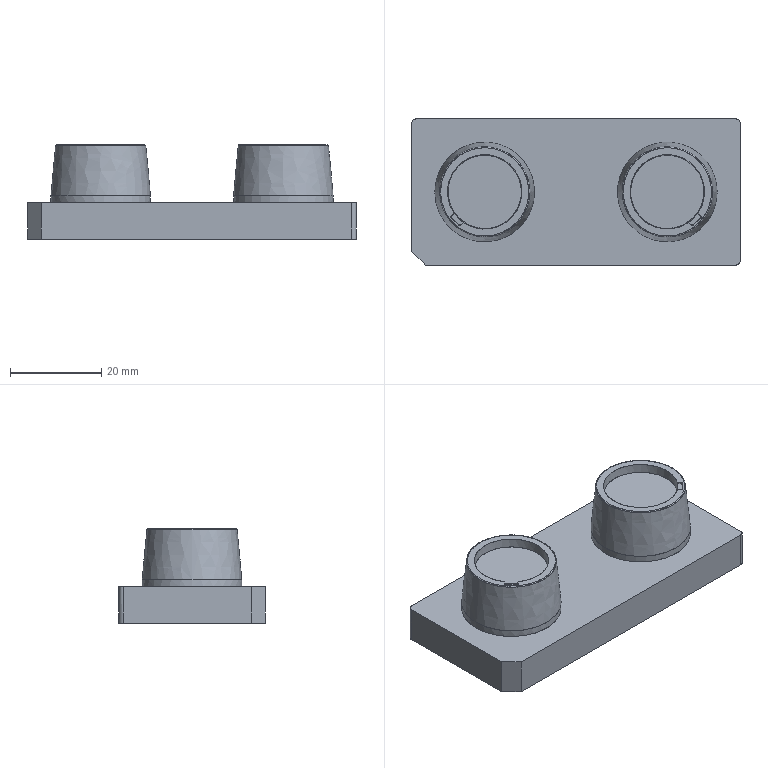NC program | PowerMill | posted with a generic post | part box 72 x 32 x 20.655 mm
Lines 24483 to 25676 of 315359:
N24580 M6
N24581 S8500 M03
N24582 G00 G90 X0.0 Y0.0
N24583 G43 Z11.805 H3
N24584
N24585 G05 P10000 R8
N24586 X-23.5434 Y-20.1661
N24587 Z0.9345
N24588 G01 Z-0.2655 F360.0
N24589 X-22.6227 Y-14.9721 F600.0
N24590 X-5.0883 Y-2.9309
N24591 X-5.0416 Y-2.7032
N24592 X-4.9592 Y-2.1939
N24593 X-4.9004 Y-1.7482
N24594 X-4.8405 Y-1.1118
N24595 X-4.8069 Y-0.4795
N24596 G03 X-4.8205 Y0.7968 I-16.4609 J0.4622
N24597 G01 X-4.8412 Y1.1159
N24598 X-4.9006 Y1.7482
N24599 X-4.9425 Y2.0766
N24600 X-4.9915 Y2.4041
N24601 X-27.6316 Y-13.1433
N24602 X-27.8712 Y-13.0029
N24603 X-28.1923 Y-12.8042
N24604 X-28.5435 Y-12.5711
N24605 X-28.8264 Y-12.374
N24606 X-29.1441 Y-12.1435
N24607 X-29.4654 Y-11.89
N24608 X-29.7833 Y-11.6323
N24609 X-30.1672 Y-11.2986
N24610 X-30.4178 Y-11.0676
N24611 X-30.7384 Y-10.7587
N24612 X-31.1708 Y-10.3051
N24613 X-6.3695 Y6.7262
N24614 X-6.4268 Y6.8444
N24615 X-6.7682 Y7.4807
N24616 X-7.1481 Y8.1163
N24617 X-7.3552 Y8.4344
N24618 X-7.5735 Y8.7524
N24619 X-7.8245 Y9.101
N24620 X-8.0467 Y9.3891
N24621 X-8.3036 Y9.7074
N24622 X-8.5753 Y10.0256
N24623 X-8.8287 Y10.306
N24624 X-33.6284 Y-6.7244
N24625 X-33.73 Y-6.523
N24626 X-33.8779 Y-6.2034
N24627 X-34.1425 Y-5.5711
N24628 X-34.2642 Y-5.252
N24629 X-34.3769 Y-4.9336
N24630 X-34.5563 Y-4.3756
N24631 X-34.7532 Y-3.6623
N24632 X-34.8275 Y-3.3423
N24633 X-34.8968 Y-3.0212
N24634 X-35.0084 Y-2.4035
N24635 X-12.3682 Y13.1439
N24636 X-12.4756 Y13.208
N24637 X-13.0644 Y13.526
N24638 X-13.5529 Y13.7649
N24639 X-13.8711 Y13.9097
N24640 X-14.1896 Y14.0457
N24641 X-14.5066 Y14.172
N24642 X-14.826 Y14.2925
N24643 X-15.145 Y14.4034
N24644 X-15.781 Y14.6032
N24645 X-16.0995 Y14.69
N24646 X-16.7366 Y14.8468
N24647 X-17.3784 Y14.9718
N24648 X-34.9156 Y2.9287
N24649 G00 Z4.0045
N24650 G01 X19.87 Y-20.4718 F10000.0
N24651 G00 Z0.9345
N24652 G01 Z-0.2655 F360.0
N24653 X19.9021 Y-15.1969 F600.0
N24654 X35.195 Y-0.4115
N24655 X35.1988 Y0.161
N24656 X35.1803 Y0.7972
N24657 X35.1585 Y1.1157
N24658 X35.0999 Y1.7525
N24659 X35.0117 Y2.3882
N24660 X34.9565 Y2.7065
N24661 X34.8735 Y3.1296
N24662 X34.7517 Y3.6605
N24663 X34.6699 Y3.9799
N24664 X34.5807 Y4.2974
N24665 X34.4825 Y4.6158
N24666 X34.4005 Y4.861
N24667 X14.657 Y-14.2273
N24668 X14.1865 Y-14.0444
N24669 X13.55 Y-13.7657
N24670 X13.0606 Y-13.5243
N24671 X12.5985 Y-13.2762
N24672 X12.2798 Y-13.0928
N24673 X11.9601 Y-12.8975
N24674 X11.6438 Y-12.6968
N24675 X11.3254 Y-12.4822
N24676 X11.0068 Y-12.2536
N24677 X10.6944 Y-12.0177
N24678 X32.3248 Y8.895
N24679 X32.1975 Y9.0709
N24680 X31.9539 Y9.3894
N24681 X31.6953 Y9.7073
N24682 X31.4242 Y10.0254
N24683 X31.1379 Y10.3444
N24684 X30.7362 Y10.758
N24685 X30.5094 Y10.9804
N24686 X30.0993 Y11.3603
N24687 X29.7809 Y11.6362
N24688 X29.4143 Y11.9352
N24689 X29.3061 Y12.0172
N24690 X7.6764 Y-8.8948
N24691 X7.3532 Y-8.4321
N24692 X7.1493 Y-8.1159
N24693 X6.8679 Y-7.6551
N24694 X6.5908 Y-7.1583
N24695 X6.2701 Y-6.5229
N24696 X6.1231 Y-6.2039
N24697 X5.9135 Y-5.7101
N24698 X5.7364 Y-5.2525
N24699 X5.5995 Y-4.862
N24700 X25.3461 Y14.2294
N24701 X25.0071 Y14.3521
N24702 X24.6222 Y14.4802
N24703 X24.3379 Y14.5676
N24704 X24.0521 Y14.6499
N24705 X23.4751 Y14.7987
N24706 X22.7788 Y14.9439
N24707 X22.1424 Y15.049
N24708 X21.5942 Y15.1165
N24709 X21.1873 Y15.1544
N24710 X20.5512 Y15.1897
N24711 X20.0996 Y15.1976
N24712 X4.8069 Y0.4124
N24713 G00 Z11.805
N24714 G05 P0
N24715 (---------------)
N24716 ( END TOOLPATH : 精公基准台01-平坦面平行-D10 )
N24717 (---------------)
N24718 ( START TOOLPATH : 精公基准台01-基准面偏置-D10 )
N24719 (---------------)
N24720 G00 X0.0 Y0.0 Z9.8045
N24721 G05 P10000 R8
N24722 X19.4876 Y26.7542
N24723 Z-11.65
N24724 G01 Z-12.85 F360.0
N24725 Y21.4792 F600.0
N24726 X19.6289 Y16.2711
N24727 X19.8415 Y16.2769
N24728 X20.4084 Y16.2725
N24729 X20.9753 Y16.2486
N24730 X21.5422 Y16.2046
N24731 X22.1091 Y16.1406
N24732 X22.676 Y16.0562
N24733 X23.2429 Y15.9513
N24734 X23.8098 Y15.8257
N24735 X24.0939 Y15.7543
N24736 X24.3767 Y15.6781
N24737 X24.9436 Y15.5089
N24738 X25.5105 Y15.3165
N24739 X25.795 Y15.2111
N24740 X26.0774 Y15.1003
N24741 X26.6443 Y14.8599
N24742 X27.2112 Y14.5934
N24743 X27.7781 Y14.2991
N24744 X28.345 Y13.9759
N24745 X28.9119 Y13.6209
N24746 X29.0863 Y13.5055
N24747 X29.4788 Y13.2332
N24748 X29.8716 Y12.9428
N24749 X30.0457 Y12.8082
N24750 X30.6126 Y12.3424
N24751 X30.8308 Y12.1503
N24752 X34.0989 Y15.6628
N24753 G02 X34.715 Y16.6625 I0.406 J0.4395
N24754 G01 X35.3022 Y16.4422
N24755 G02 X36.0814 Y15.775 I-0.5263 J-1.4033
N24756 G01 X36.5893 Y14.8742
N24757 G02 X35.6331 Y14.16 I-0.5241 J-0.2955
N24758 G01 X35.1846 Y14.6229
N24759 X34.7212 Y15.0839
N24760 X34.0989 Y15.6628
N24761 X30.8308 Y12.1503
N24762 X31.1945 Y11.8173
N24763 X31.4705 Y11.5492
N24764 X31.76 Y11.2546
N24765 X32.0231 Y10.9732
N24766 X32.3133 Y10.6463
N24767 X32.7421 Y10.1291
N24768 X32.8802 Y9.953
N24769 X33.1698 Y9.5664
N24770 X33.4471 Y9.1727
N24771 X33.5606 Y9.0037
N24772 X33.918 Y8.441
N24773 X34.014 Y8.2805
N24774 X34.2441 Y7.8782
N24775 X34.581 Y7.2358
N24776 X34.811 Y6.7528
N24777 X35.0548 Y6.19
N24778 X35.1669 Y5.9096
N24779 X35.2741 Y5.6273
N24780 X35.4698 Y5.0646
N24781 X35.6425 Y4.5018
N24782 X35.7208 Y4.2212
N24783 X35.7939 Y3.9391
N24784 X35.9235 Y3.3764
N24785 X36.0328 Y2.8137
N24786 X36.1214 Y2.2509
N24787 X36.19 Y1.6882
N24788 X36.2387 Y1.1255
N24789 X36.2681 Y0.5627
N24790 X36.2778 Y0.0
N24791 X36.2681 Y-0.5627
N24792 X36.2387 Y-1.1255
N24793 X36.19 Y-1.6882
N24794 X36.1214 Y-2.2509
N24795 X36.0328 Y-2.8137
N24796 X35.9235 Y-3.3764
N24797 X35.7939 Y-3.9391
N24798 X35.7208 Y-4.2212
N24799 X35.6425 Y-4.5018
N24800 X35.4698 Y-5.0646
N24801 X35.2741 Y-5.6273
N24802 X35.1669 Y-5.9096
N24803 X35.0548 Y-6.19
N24804 X34.811 Y-6.7528
N24805 X34.5411 Y-7.3155
N24806 X34.2441 Y-7.8782
N24807 X34.014 Y-8.2805
N24808 X33.918 Y-8.441
N24809 X33.5606 Y-9.0037
N24810 X33.4471 Y-9.1727
N24811 X33.1698 Y-9.5664
N24812 X32.8802 Y-9.953
N24813 X32.7421 Y-10.1291
N24814 X32.2738 Y-10.6919
N24815 X32.1619 Y-10.8175
N24816 X35.6316 Y-14.1542
N24817 G02 X36.6124 Y-14.8059 I0.4313 J-0.4148
N24818 G01 X36.3455 Y-15.4249
N24819 G02 X36.0958 Y-15.8122 I-1.2842 J0.5536
N24820 G01 X35.901 Y-16.0264
N24821 G02 X35.3871 Y-16.3834 I-1.0346 J0.9409
N24822 G01 X34.7924 Y-16.622
N24823 G02 X34.1531 Y-15.6327 I-0.2234 J0.5569
N24824 G01 X34.6302 Y-15.1738
N24825 X35.1735 Y-14.6306
N24826 X35.6316 Y-14.1542
N24827 X32.1619 Y-10.8175
N24828 X32.0231 Y-10.9732
N24829 X31.76 Y-11.2546
N24830 X31.4705 Y-11.5494
N24831 X31.1945 Y-11.8173
N24832 X30.8961 Y-12.0929
N24833 X30.5686 Y-12.3801
N24834 X30.0457 Y-12.8082
N24835 X29.8716 Y-12.9428
N24836 X29.4788 Y-13.2332
N24837 X29.0863 Y-13.5055
N24838 X28.9119 Y-13.6209
N24839 X28.345 Y-13.9759
N24840 X27.7781 Y-14.2991
N24841 X27.1343 Y-14.631
N24842 X26.6443 Y-14.8599
N24843 X26.0774 Y-15.1003
N24844 X25.795 Y-15.2111
N24845 X25.5105 Y-15.3165
N24846 X24.9436 Y-15.5089
N24847 X24.3767 Y-15.6781
N24848 X24.0939 Y-15.7543
N24849 X23.8098 Y-15.8257
N24850 X23.2429 Y-15.9513
N24851 X22.676 Y-16.0562
N24852 X22.1091 Y-16.1406
N24853 X21.5422 Y-16.2046
N24854 X20.9753 Y-16.2486
N24855 X20.4084 Y-16.2725
N24856 X19.8415 Y-16.2769
N24857 X19.2746 Y-16.2615
N24858 X18.7077 Y-16.2263
N24859 X18.1408 Y-16.1711
N24860 X17.5739 Y-16.0958
N24861 X17.007 Y-16.0002
N24862 X16.4401 Y-15.8837
N24863 X15.8732 Y-15.746
N24864 X15.3063 Y-15.5864
N24865 X14.7394 Y-15.4042
N24866 X14.1725 Y-15.1989
N24867 X13.6056 Y-14.969
N24868 X13.0387 Y-14.714
N24869 X12.866 Y-14.631
N24870 X12.4718 Y-14.4323
N24871 X11.8119 Y-14.0683
N24872 X11.338 Y-13.7817
N24873 X10.9137 Y-13.5055
N24874 X10.7711 Y-13.408
N24875 X10.1284 Y-12.9428
N24876 X9.6373 Y-12.5529
N24877 X9.4314 Y-12.3801
N24878 X9.1926 Y-12.1701
N24879 X5.8526 Y-15.6353
N24880 G02 X5.4332 Y-16.6748 I-0.4194 J-0.4351
N24881 G01 X-5.4269 Y-16.6749
N24882 G02 X-5.8475 Y-15.6348 I0.0 J0.6051
N24883 G01 X-5.3431 Y-15.1471
N24884 G03 X-0.8619 Y-8.8312 I-14.6234 J15.1234
N24885 G01 X-0.564 Y-8.1852
N24886 G02 X0.5632 Y-8.1855 I0.5635 J-0.2598
N24887 G01 X0.8604 Y-8.8311
N24888 G03 X5.3482 Y-15.1491 I19.0154 J8.754
N24889 G01 X5.8526 Y-15.6353
N24890 X9.1926 Y-12.1701
N24891 X9.0704 Y-12.0627
N24892 X8.8055 Y-11.8173
N24893 X8.5035 Y-11.5236
N24894 X8.24 Y-11.2546
N24895 X7.9366 Y-10.9287
N24896 X7.7262 Y-10.6919
N24897 X7.3697 Y-10.2685
N24898 X7.0389 Y-9.8478
N24899 X6.8028 Y-9.5288
N24900 X6.4394 Y-9.0037
N24901 X6.2359 Y-8.6896
N24902 X6.082 Y-8.441
N24903 X5.7556 Y-7.8782
N24904 X5.4586 Y-7.3155
N24905 X5.189 Y-6.7528
N24906 X4.9452 Y-6.19
N24907 X4.7262 Y-5.6273
N24908 X4.5302 Y-5.0646
N24909 X4.3572 Y-4.5018
N24910 X4.2061 Y-3.9391
N24911 X4.0768 Y-3.3764
N24912 X3.9672 Y-2.8137
N24913 X3.8786 Y-2.2509
N24914 X3.8102 Y-1.6882
N24915 X3.7613 Y-1.1255
N24916 X3.7319 Y-0.5627
N24917 X3.7222 Y0.0
N24918 X3.7319 Y0.5627
N24919 X3.7613 Y1.1255
N24920 X3.8102 Y1.6882
N24921 X3.8786 Y2.2509
N24922 X3.9672 Y2.8137
N24923 X4.0768 Y3.3764
N24924 X4.2061 Y3.9391
N24925 X4.3572 Y4.5018
N24926 X4.5302 Y5.0646
N24927 X4.7262 Y5.6273
N24928 X4.9452 Y6.19
N24929 X5.189 Y6.7528
N24930 X5.4586 Y7.3155
N24931 X5.7556 Y7.8782
N24932 X6.082 Y8.441
N24933 X6.2359 Y8.6896
N24934 X6.4394 Y9.0037
N24935 X6.8028 Y9.5288
N24936 X7.0389 Y9.8478
N24937 X7.3697 Y10.2685
N24938 X7.7262 Y10.6919
N24939 X7.9366 Y10.9287
N24940 X8.24 Y11.2546
N24941 X8.5035 Y11.5236
N24942 X8.8055 Y11.8173
N24943 X9.0704 Y12.0627
N24944 X9.4314 Y12.3801
N24945 X9.6373 Y12.5529
N24946 X10.2042 Y13.0002
N24947 X10.7711 Y13.408
N24948 X10.9137 Y13.5055
N24949 X11.338 Y13.7817
N24950 X11.9049 Y14.1221
N24951 X12.4718 Y14.4323
N24952 X12.866 Y14.631
N24953 X13.0387 Y14.714
N24954 X13.6056 Y14.969
N24955 X14.1725 Y15.1989
N24956 X14.7394 Y15.4042
N24957 X15.3063 Y15.5864
N24958 X15.9139 Y15.7565
N24959 X16.4401 Y15.8837
N24960 X17.007 Y16.0002
N24961 X17.5739 Y16.0958
N24962 X18.1408 Y16.1711
N24963 X18.7077 Y16.2263
N24964 X19.2746 Y16.2615
N24965 X19.6289 Y16.2711
N24966 X19.4876 Y21.4792
N24967 G00 Z2.9153
N24968 G01 X-19.4875 Y-26.7548 F10000.0
N24969 G00 Z-11.65
N24970 G01 Z-12.85 F360.0
N24971 X-19.4876 Y-21.4798 F600.0
N24972 X-19.6289 Y-16.2711
N24973 X-19.8415 Y-16.2769
N24974 X-20.4084 Y-16.2725
N24975 X-20.9753 Y-16.2486
N24976 X-21.5422 Y-16.2046
N24977 X-22.1091 Y-16.1406
N24978 X-22.676 Y-16.0562
N24979 X-23.2429 Y-15.9513
N24980 X-23.8098 Y-15.8257
N24981 X-24.0858 Y-15.7565
N24982 X-24.3767 Y-15.6781
N24983 X-24.9436 Y-15.5089
N24984 X-25.5105 Y-15.3165
N24985 X-25.795 Y-15.2111
N24986 X-26.0774 Y-15.1003
N24987 X-26.6443 Y-14.8599
N24988 X-27.2112 Y-14.5934
N24989 X-27.7781 Y-14.2991
N24990 X-28.345 Y-13.9759
N24991 X-28.9119 Y-13.6209
N24992 X-29.0863 Y-13.5055
N24993 X-29.4788 Y-13.2332
N24994 X-29.8716 Y-12.9428
N24995 X-30.0457 Y-12.8082
N24996 X-30.6126 Y-12.3424
N24997 X-30.8961 Y-12.0929
N24998 X-31.1945 Y-11.8173
N24999 X-31.4705 Y-11.5494
N25000 X-31.76 Y-11.2546
N25001 X-32.0231 Y-10.9732
N25002 X-32.3133 Y-10.6463
N25003 X-32.7421 Y-10.1291
N25004 X-32.8802 Y-9.953
N25005 X-33.1698 Y-9.5664
N25006 X-33.4471 Y-9.1727
N25007 X-33.5606 Y-9.0037
N25008 X-33.918 Y-8.441
N25009 X-34.014 Y-8.2805
N25010 X-34.2441 Y-7.8782
N25011 X-34.581 Y-7.2358
N25012 X-34.811 Y-6.7528
N25013 X-35.0548 Y-6.19
N25014 X-35.1669 Y-5.9096
N25015 X-35.2741 Y-5.6273
N25016 X-35.4698 Y-5.0646
N25017 X-35.6425 Y-4.5018
N25018 X-35.7208 Y-4.2212
N25019 X-35.7939 Y-3.9391
N25020 X-35.9235 Y-3.3764
N25021 X-36.0328 Y-2.8137
N25022 X-36.1214 Y-2.2509
N25023 X-36.19 Y-1.6882
N25024 X-36.2387 Y-1.1255
N25025 X-36.2681 Y-0.5627
N25026 X-36.2778 Y0.0
N25027 X-36.2681 Y0.5627
N25028 X-36.2387 Y1.1255
N25029 X-36.19 Y1.6882
N25030 X-36.1214 Y2.2509
N25031 X-36.0328 Y2.8137
N25032 X-35.9235 Y3.3764
N25033 X-35.7939 Y3.9391
N25034 X-35.7208 Y4.2212
N25035 X-35.6425 Y4.5018
N25036 X-35.4698 Y5.0646
N25037 X-35.2741 Y5.6273
N25038 X-35.1669 Y5.9096
N25039 X-35.0548 Y6.19
N25040 X-34.811 Y6.7528
N25041 X-34.5411 Y7.3155
N25042 X-34.2441 Y7.8782
N25043 X-34.014 Y8.2805
N25044 X-33.918 Y8.441
N25045 X-33.5606 Y9.0037
N25046 X-33.4471 Y9.1727
N25047 X-33.1698 Y9.5664
N25048 X-32.8802 Y9.953
N25049 X-32.7421 Y10.1291
N25050 X-32.2738 Y10.6919
N25051 X-32.1621 Y10.8172
N25052 X-35.6317 Y14.1539
N25053 G02 X-36.5873 Y14.8566 I-0.4312 J0.4147
N25054 G01 X-36.092 Y15.7583
N25055 G02 X-35.3869 Y16.383 I1.2258 J-0.6732
N25056 G01 X-34.7924 Y16.6215
N25057 G02 X-34.1532 Y15.6325 I0.2234 J-0.5567
N25058 G01 X-34.6303 Y15.1736
N25059 X-35.1736 Y14.6303
N25060 X-35.6317 Y14.1539
N25061 X-32.1621 Y10.8172
N25062 X-32.0231 Y10.9732
N25063 X-31.76 Y11.2546
N25064 X-31.4705 Y11.5492
N25065 X-31.1945 Y11.8173
N25066 X-30.8961 Y12.0929
N25067 X-30.5686 Y12.3801
N25068 X-30.0457 Y12.8082
N25069 X-29.8716 Y12.9428
N25070 X-29.4788 Y13.2332
N25071 X-29.0863 Y13.5055
N25072 X-28.9119 Y13.6209
N25073 X-28.345 Y13.9759
N25074 X-27.7781 Y14.2991
N25075 X-27.1343 Y14.631
N25076 X-26.6443 Y14.8599
N25077 X-26.0774 Y15.1003
N25078 X-25.795 Y15.2111
N25079 X-25.5105 Y15.3165
N25080 X-24.9436 Y15.5089
N25081 X-24.3767 Y15.6781
N25082 X-24.0939 Y15.7543
N25083 X-23.8098 Y15.8257
N25084 X-23.2429 Y15.9513
N25085 X-22.676 Y16.0562
N25086 X-22.1091 Y16.1406
N25087 X-21.5422 Y16.2046
N25088 X-20.9753 Y16.2486
N25089 X-20.4084 Y16.2725
N25090 X-19.8415 Y16.2769
N25091 X-19.2746 Y16.2615
N25092 X-18.7077 Y16.2263
N25093 X-18.1408 Y16.1711
N25094 X-17.5739 Y16.0958
N25095 X-17.007 Y16.0002
N25096 X-16.4401 Y15.8837
N25097 X-15.8732 Y15.746
N25098 X-15.3063 Y15.5864
N25099 X-14.7394 Y15.4042
N25100 X-14.1725 Y15.1989
N25101 X-13.6056 Y14.969
N25102 X-13.0387 Y14.714
N25103 X-12.866 Y14.631
N25104 X-12.4718 Y14.4323
N25105 X-11.8119 Y14.0683
N25106 X-11.338 Y13.7817
N25107 X-10.9137 Y13.5055
N25108 X-10.7711 Y13.408
N25109 X-10.1284 Y12.9428
N25110 X-9.6373 Y12.5529
N25111 X-9.4314 Y12.3801
N25112 X-9.1923 Y12.1699
N25113 X-5.8522 Y15.6349
N25114 G02 X-5.4328 Y16.6745 I0.4194 J0.4352
N25115 G01 X5.4262
N25116 G02 X5.8462 Y15.6338 I0.0 J-0.6051
N25117 G01 X5.3706 Y15.1752
N25118 G03 X1.6996 Y10.4573 I14.6205 J-15.1634
N25119 G01 X1.6848 Y10.4314
N25120 G03 X0.8501 Y8.8076 I18.0129 J-10.2864
N25121 G01 X0.5643 Y8.1858
N25122 G02 X-0.5632 Y8.1855 I-0.5638 J0.2592
N25123 G01 X-0.8605 Y8.8312
N25124 G03 X-5.3478 Y15.1488 I-19.0152 J-8.754
N25125 G01 X-5.8522 Y15.6349
N25126 X-9.1923 Y12.1699
N25127 X-9.0704 Y12.0627
N25128 X-8.8055 Y11.8173
N25129 X-8.5035 Y11.5236
N25130 X-8.24 Y11.2546
N25131 X-7.9366 Y10.9287
N25132 X-7.7262 Y10.6919
N25133 X-7.3697 Y10.2685
N25134 X-7.0388 Y9.8478
N25135 X-6.8028 Y9.5288
N25136 X-6.4394 Y9.0037
N25137 X-6.2359 Y8.6896
N25138 X-6.082 Y8.441
N25139 X-5.7556 Y7.8782
N25140 X-5.4586 Y7.3155
N25141 X-5.189 Y6.7528
N25142 X-4.9452 Y6.19
N25143 X-4.7262 Y5.6273
N25144 X-4.5302 Y5.0646
N25145 X-4.3572 Y4.5018
N25146 X-4.2061 Y3.9391
N25147 X-4.0768 Y3.3764
N25148 X-3.9672 Y2.8137
N25149 X-3.8786 Y2.2509
N25150 X-3.8102 Y1.6882
N25151 X-3.7613 Y1.1255
N25152 X-3.7319 Y0.5627
N25153 X-3.7222 Y0.0
N25154 X-3.7319 Y-0.5627
N25155 X-3.7613 Y-1.1255
N25156 X-3.8102 Y-1.6882
N25157 X-3.8786 Y-2.2509
N25158 X-3.9672 Y-2.8137
N25159 X-4.0768 Y-3.3764
N25160 X-4.2061 Y-3.9391
N25161 X-4.3572 Y-4.5018
N25162 X-4.5302 Y-5.0646
N25163 X-4.7262 Y-5.6273
N25164 X-4.9452 Y-6.19
N25165 X-5.189 Y-6.7528
N25166 X-5.4586 Y-7.3155
N25167 X-5.7556 Y-7.8782
N25168 X-6.082 Y-8.441
N25169 X-6.2359 Y-8.6896
N25170 X-6.4394 Y-9.0037
N25171 X-6.8028 Y-9.5288
N25172 X-7.0388 Y-9.8478
N25173 X-7.3697 Y-10.2685
N25174 X-7.7262 Y-10.6919
N25175 X-7.9366 Y-10.9287
N25176 X-8.24 Y-11.2546
N25177 X-8.5035 Y-11.5236
N25178 X-8.8055 Y-11.8173
N25179 X-9.0704 Y-12.0627
N25180 X-9.4314 Y-12.3801
N25181 X-9.6373 Y-12.5529
N25182 X-10.2042 Y-13.0002
N25183 X-10.7711 Y-13.408
N25184 X-10.9137 Y-13.5055
N25185 X-11.338 Y-13.7817
N25186 X-11.9049 Y-14.1221
N25187 X-12.4718 Y-14.4323
N25188 X-12.866 Y-14.631
N25189 X-13.0387 Y-14.714
N25190 X-13.6056 Y-14.969
N25191 X-14.1725 Y-15.1989
N25192 X-14.7394 Y-15.4042
N25193 X-15.3063 Y-15.5864
N25194 X-15.9139 Y-15.7565
N25195 X-16.4401 Y-15.8837
N25196 X-17.007 Y-16.0002
N25197 X-17.5739 Y-16.0958
N25198 X-18.1408 Y-16.1711
N25199 X-18.7077 Y-16.2263
N25200 X-19.2746 Y-16.2615
N25201 X-19.6289 Y-16.2711
N25202 X-19.4876 Y-21.4798
N25203 G00 Z9.8045
N25204 G05 P0
N25205 (---------------)
N25206 ( END TOOLPATH : 精公基准台01-基准面偏置-D10 )
N25207 (---------------)
N25208 ( START TOOLPATH : 精公基准台01-外形侧光-D10 )
N25209 (---------------)
N25210 G00 X0.0 Y0.0 Z10.805
N25211 G05 P10000 R8
N25212 X-7.7008 Y-10.8216
N25213 Z-11.62
N25214 G01 Z-12.82 F360.0
N25215 G03 X-8.762 Y-11.2598 I-0.0017 J-1.5 F600.0
N25216 G02 X-12.6512 Y-14.1084 I-11.2343 J11.259
N25217 G02 X-26.1311 Y14.6786 I-7.3486 J14.1085
N25218 G02 X-13.0177 Y14.2918 I6.13 J-14.6615
N25219 G02 X-8.762 Y-11.2598 I-6.9786 J-14.2925
N25220 G03 X-9.2025 Y-12.32 I1.0595 J-1.0618
N25221 G01 X-7.7577 Y-10.7654
N25222 G03 X-8.8189 Y-11.2036 I-0.0017 J-1.5
N25223 G02 X-12.6877 Y-14.0372 I-11.1774 J11.2029
N25224 G02 X-26.1009 Y14.6045 I-7.3121 J14.0373
N25225 G02 X-13.0528 Y14.2199 I6.0998 J-14.5874
N25226 G02 X-8.8189 Y-11.2036 I-6.9435 J-14.2206
N25227 G03 X-9.2594 Y-12.2637 I1.0595 J-1.0618
N25228 G00 Z3.8889
N25229 G01 X32.3051 Y-10.8135 F10000.0
N25230 G00 Z-11.62
N25231 G01 Z-12.82 F360.0
N25232 G03 X31.2442 Y-11.2524 I-0.0006 J-1.5 F600.0
N25233 G02 X5.367 Y6.239 I-11.2442 J11.2525
N25234 G02 X5.3873 Y6.2866 I14.4728 J-6.1706
N25235 G02 X34.0162 Y-7.523 I14.6126 J-6.2867
N25236 G02 X31.2442 Y-11.2524 I-14.0162 J7.5231
N25237 G03 X30.8045 Y-12.3129 I1.0603 J-1.0611
N25238 G01 X32.2485 Y-10.7569
N25239 G03 X31.1877 Y-11.1958 I-0.0006 J-1.5
N25240 G02 X5.4402 Y6.2069 I-11.1877 J11.1959
N25241 G02 X5.4608 Y6.255 I14.4168 J-6.1458
N25242 G02 X33.9459 Y-7.4848 I14.5391 J-6.2551
N25243 G02 X31.1877 Y-11.1958 I-13.9459 J7.4849
N25244 G03 X30.7479 Y-12.2563 I1.0603 J-1.0611
N25245 G00 Z10.805
N25246 G05 P0
N25247 (---------------)
N25248 ( END TOOLPATH : 精公基准台01-外形侧光-D10 )
N25249 (---------------)
N25250 ( START TOOLPATH : 精公基准台01-基准台侧光-D10 )
N25251 (---------------)
N25252 G00 X0.0 Y0.0 Z9.8045
N25253 G05 P10000 R8
N25254 X41.3737 Y-24.0629
N25255 Z-19.55
N25256 G01 Z-20.75 F360.0
N25257 G03 X38.4836 Y-19.9828 I-1.4451 J2.04 F600.0
N25258 G01 X38.4835 Y-19.9829
N25259 X38.4825 Y-19.9836
N25260 X38.2982 Y-20.1073
N25261 X38.2966 Y-20.1083
N25262 X38.295 Y-20.1093
N25263 X37.9788 Y-20.3001
N25264 X37.9767 Y-20.3014
N25265 X37.9746 Y-20.3025
N25266 X37.6584 Y-20.468
N25267 X37.6563 Y-20.469
N25268 X37.6542 Y-20.47
N25269 X37.338 Y-20.6125
N25270 X37.3359 Y-20.6134
N25271 X37.3338 Y-20.6142
N25272 X37.0177 Y-20.7354
N25273 X37.0156 Y-20.7361
N25274 X37.0135 Y-20.7368
N25275 X36.6973 Y-20.8382
N25276 X36.6952 Y-20.8389
N25277 X36.6931 Y-20.8395
N25278 X36.377 Y-20.922
N25279 X36.3756 Y-20.9224
N25280 X36.3742 Y-20.9227
N25281 X36.2802 Y-20.9437
N25282 X36.2791 Y-20.9439
N25283 X36.2779 Y-20.9442
N25284 X36.0557 Y-20.9869
N25285 X36.0541 Y-20.9872
N25286 X36.0525 Y-20.9875
N25287 X35.7364 Y-21.0352
N25288 X35.7341 Y-21.0355
N25289 X35.7318 Y-21.0357
N25290 X35.4157 Y-21.065
N25291 X35.4138 Y-21.0652
N25292 X35.4118 Y-21.0653
N25293 X35.0957 Y-21.0791
N25294 X35.094
N25295 X35.0924 Y-21.0792
N25296 X34.7762 Y-21.08
N25297 X34.7761
N25298 X34.776
N25299 X-32.8792
N25300 X-32.8796
N25301 X-32.8801
N25302 X-33.1963 Y-21.0762
N25303 X-33.1986 Y-21.0761
N25304 X-33.201 Y-21.076
N25305 X-33.5171 Y-21.0536
N25306 X-33.5196 Y-21.0534
N25307 X-33.5222 Y-21.0531
N25308 X-33.8383 Y-21.0103
N25309 X-33.8408 Y-21.0099
N25310 X-33.8434 Y-21.0095
N25311 X-34.1595 Y-20.9459
N25312 X-34.162 Y-20.9453
N25313 X-34.1646 Y-20.9447
N25314 X-34.4807 Y-20.8594
N25315 X-34.4833 Y-20.8586
N25316 X-34.4858 Y-20.8578
N25317 X-34.8019 Y-20.7496
N25318 X-34.8044 Y-20.7487
N25319 X-34.8068 Y-20.7478
N25320 X-35.105 Y-20.6233
N25321 X-35.1076 Y-20.6222
N25322 X-35.1101 Y-20.621
N25323 X-35.4442 Y-20.4533
N25324 X-35.4468 Y-20.4519
N25325 X-35.4494 Y-20.4504
N25326 X-35.7656 Y-20.2612
N25327 X-35.7681 Y-20.2596
N25328 X-35.7706 Y-20.2579
N25329 X-36.0868 Y-20.0346
N25330 X-36.0883 Y-20.0335
N25331 X-36.0898 Y-20.0323
N25332 X-36.1566 Y-19.9803
N25333 X-36.1579 Y-19.9792
N25334 X-36.1591 Y-19.9782
N25335 X-36.4085 Y-19.7667
N25336 X-36.4099 Y-19.7655
N25337 X-36.4114 Y-19.7642
N25338 X-36.5234 Y-19.6595
N25339 X-36.5243 Y-19.6586
N25340 X-36.5252 Y-19.6578
N25341 X-36.7293 Y-19.4549
N25342 X-36.7294 Y-19.4548
N25343 X-36.7295 Y-19.4547
N25344 X-39.5748 Y-16.6094
N25345 X-39.5751 Y-16.6091
N25346 X-39.5754 Y-16.6088
N25347 X-39.6862 Y-16.4955
N25348 X-39.6875 Y-16.4942
N25349 X-39.6887 Y-16.4928
N25350 X-39.8941 Y-16.2622
N25351 X-39.8952 Y-16.261
N25352 X-39.8963 Y-16.2597
N25353 X-39.9663 Y-16.1741
N25354 X-39.9676 Y-16.1725
N25355 X-39.9688 Y-16.1709
N25356 X-40.2019 Y-15.8548
N25357 X-40.2037 Y-15.8523
N25358 X-40.2054 Y-15.8497
N25359 X-40.4031 Y-15.5336
N25360 X-40.4046 Y-15.531
N25361 X-40.406 Y-15.5285
N25362 X-40.5729 Y-15.2123
N25363 X-40.5742 Y-15.2098
N25364 X-40.5754 Y-15.2073
N25365 X-40.7148 Y-14.8911
N25366 X-40.7159 Y-14.8886
N25367 X-40.7169 Y-14.8861
N25368 X-40.8313 Y-14.5699
N25369 X-40.8322 Y-14.5674
N25370 X-40.8329 Y-14.5649
N25371 X-40.9241 Y-14.2487
N25372 X-40.9248 Y-14.2462
N25373 X-40.9254 Y-14.2437
N25374 X-40.9946 Y-13.9275
N25375 X-40.9951 Y-13.925
N25376 X-40.9955 Y-13.9225
N25377 X-41.0437 Y-13.6063
N25378 X-41.044 Y-13.6038
N25379 X-41.0443 Y-13.6012
N25380 X-41.072 Y-13.2851
N25381 X-41.0721 Y-13.2826
N25382 X-41.0722 Y-13.2801
N25383 X-41.08 Y-12.9639
N25384 Y-12.963
N25385 Y-12.962
N25386 Y14.8588
N25387 Y14.8592
N25388 Y14.8596
N25389 X-41.077 Y15.1758
N25390 X-41.0769 Y15.1775
N25391 X-41.0768 Y15.1793
N25392 X-41.0597 Y15.4955
N25393 X-41.0596 Y15.4976
N25394 X-41.0594 Y15.4998
N25395 X-41.025 Y15.8159
N25396 X-41.0247 Y15.8181
N25397 X-41.0244 Y15.8202
N25398 X-40.9728 Y16.1363
N25399 X-40.9724 Y16.1384
N25400 X-40.972 Y16.1405
N25401 X-40.9029 Y16.4567
N25402 X-40.9024 Y16.4588
N25403 X-40.9018 Y16.4609
N25404 X-40.8145 Y16.777
N25405 X-40.8139 Y16.7792
N25406 X-40.8132 Y16.7814
N25407 X-40.7061 Y17.0975
N25408 X-40.7054 Y17.0995
N25409 X-40.7046 Y17.1015
N25410 X-40.5786 Y17.4176
N25411 X-40.5776 Y17.4199
N25412 X-40.5766 Y17.4221
N25413 X-40.4277 Y17.7383
N25414 X-40.4267 Y17.7402
N25415 X-40.4257 Y17.7422
N25416 X-40.2547 Y18.0584
N25417 X-40.2535 Y18.0605
N25418 X-40.2522 Y18.0627
N25419 X-40.0546 Y18.3788
N25420 X-40.0535 Y18.3806
N25421 X-40.0523 Y18.3824
N25422 X-39.8998 Y18.5997
N25423 X-39.8991 Y18.6007
N25424 X-39.8983 Y18.6018
N25425 X-39.8241 Y18.7006
N25426 X-39.823 Y18.702
N25427 X-39.822 Y18.7033
N25428 X-39.5801 Y18.9986
N25429 X-39.5783 Y19.0007
N25430 X-39.5764 Y19.0028
N25431 X-39.2602 Y19.3377
N25432 X-39.2581 Y19.3398
N25433 X-39.256 Y19.3419
N25434 X-38.9398 Y19.6301
N25435 X-38.9378 Y19.6319
N25436 X-38.9357 Y19.6336
N25437 X-38.6196 Y19.8851
N25438 X-38.618 Y19.8863
N25439 X-38.6164 Y19.8875
N25440 X-38.4845 Y19.9822
N25441 X-38.4835 Y19.9829
N25442 X-38.4825 Y19.9836
N25443 X-38.2982 Y20.1073
N25444 X-38.2966 Y20.1083
N25445 X-38.295 Y20.1093
N25446 X-37.9788 Y20.3001
N25447 X-37.9767 Y20.3014
N25448 X-37.9746 Y20.3025
N25449 X-37.6584 Y20.468
N25450 X-37.6563 Y20.469
N25451 X-37.6542 Y20.47
N25452 X-37.338 Y20.6125
N25453 X-37.3359 Y20.6134
N25454 X-37.3338 Y20.6142
N25455 X-37.0177 Y20.7354
N25456 X-37.0156 Y20.7361
N25457 X-37.0135 Y20.7368
N25458 X-36.6973 Y20.8382
N25459 X-36.6952 Y20.8389
N25460 X-36.6931 Y20.8395
N25461 X-36.377 Y20.922
N25462 X-36.3748 Y20.9225
N25463 X-36.3726 Y20.923
N25464 X-36.0564 Y20.9868
N25465 X-36.0545 Y20.9871
N25466 X-36.0525 Y20.9875
N25467 X-35.7364 Y21.0352
N25468 X-35.7341 Y21.0355
N25469 X-35.7318 Y21.0357
N25470 X-35.4157 Y21.065
N25471 X-35.4138 Y21.0652
N25472 X-35.4118 Y21.0653
N25473 X-35.0957 Y21.0791
N25474 X-35.094
N25475 X-35.0924 Y21.0792
N25476 X-34.7762 Y21.08
N25477 X-34.7761
N25478 X-34.776
N25479 X0.0
N25480 X34.776
N25481 X34.7761
N25482 X34.7762
N25483 X35.0924 Y21.0792
N25484 X35.0939 Y21.0791
N25485 X35.0955
N25486 X35.4116 Y21.066
N25487 X35.4137 Y21.0659
N25488 X35.4159 Y21.0657
N25489 X35.732 Y21.0357
N25490 X35.7341 Y21.0355
N25491 X35.7362 Y21.0352
N25492 X36.0524 Y20.9882
N25493 X36.0545 Y20.9879
N25494 X36.0566 Y20.9875
N25495 X36.3727 Y20.923
N25496 X36.3749 Y20.9225
N25497 X36.377 Y20.922
N25498 X36.6931 Y20.8394
N25499 X36.6952 Y20.8388
N25500 X36.6973 Y20.8382
N25501 X37.0135 Y20.7367
N25502 X37.0155 Y20.736
N25503 X37.0175 Y20.7353
N25504 X37.3095 Y20.6242
N25505 X37.3117 Y20.6234
N25506 X37.3138 Y20.6225
N25507 X37.6541 Y20.4699
N25508 X37.6562 Y20.4689
N25509 X37.6584 Y20.4678
N25510 X37.9715 Y20.3042
N25511 X37.9737 Y20.3031
N25512 X37.9758 Y20.3018
N25513 X38.2949 Y20.1096
N25514 X38.2966 Y20.1085
N25515 X38.2982 Y20.1075
N25516 X38.4828 Y19.9836
N25517 X38.4839 Y19.9829
N25518 X38.485 Y19.9821
N25519 X38.6165 Y19.8874
N25520 X38.6179 Y19.8864
N25521 X38.6193 Y19.8853
N25522 X38.9005 Y19.6639
N25523 X38.9027 Y19.6621
N25524 X38.9048 Y19.6603
N25525 X39.2536 Y19.3442
N25526 X39.2558 Y19.3421
N25527 X39.2579 Y19.3399
N25528 X39.5579 Y19.0238
N25529 X39.5598 Y19.0217
N25530 X39.5616 Y19.0196
N25531 X39.8219 Y18.7034
N25532 X39.823 Y18.702
N25533 X39.8241 Y18.7006
N25534 X39.8983 Y18.6018
N25535 X39.8992 Y18.6006
N25536 X39.9 Y18.5994
N25537 X40.0514 Y18.3822
N25538 X40.0523 Y18.3808
N25539 X40.0532 Y18.3794
N25540 X40.218 Y18.1205
N25541 X40.2193 Y18.1184
N25542 X40.2206 Y18.1162
N25543 X40.4261 Y17.7427
N25544 X40.4273 Y17.7404
N25545 X40.4285 Y17.7381
N25546 X40.5767 Y17.422
N25547 X40.5776 Y17.4199
N25548 X40.5785 Y17.4178
N25549 X40.7052 Y17.1016
N25550 X40.706 Y17.0995
N25551 X40.7068 Y17.0974
N25552 X40.8132 Y16.7812
N25553 X40.8138 Y16.7791
N25554 X40.8144 Y16.777
N25555 X40.9018 Y16.4609
N25556 X40.9023 Y16.4588
N25557 X40.9028 Y16.4566
N25558 X40.9718 Y16.1405
N25559 X40.9722 Y16.1384
N25560 X40.9726 Y16.1364
N25561 X41.0244 Y15.8202
N25562 X41.0247 Y15.8181
N25563 X41.025 Y15.8159
N25564 X41.0591 Y15.4997
N25565 X41.0593 Y15.4976
N25566 X41.0595 Y15.4955
N25567 X41.0768 Y15.1794
N25568 X41.0769 Y15.1776
N25569 Y15.1758
N25570 X41.08 Y14.8596
N25571 Y14.8592
N25572 Y14.8588
N25573 Y-14.8588
N25574 Y-14.8592
N25575 Y-14.8596
N25576 X41.077 Y-15.1758
N25577 X41.0769 Y-15.1775
N25578 X41.0768 Y-15.1793
N25579 X41.0598 Y-15.4955
N25580 X41.0596 Y-15.4976
N25581 X41.0594 Y-15.4998
N25582 X41.025 Y-15.8159
N25583 X41.0247 Y-15.8181
N25584 X41.0244 Y-15.8202
N25585 X40.9728 Y-16.1363
N25586 X40.9724 Y-16.1384
N25587 X40.972 Y-16.1405
N25588 X40.9029 Y-16.4567
N25589 X40.9024 Y-16.4588
N25590 X40.9018 Y-16.4609
N25591 X40.8145 Y-16.777
N25592 X40.8139 Y-16.7792
N25593 X40.8132 Y-16.7814
N25594 X40.7061 Y-17.0975
N25595 X40.7054 Y-17.0995
N25596 X40.7046 Y-17.1015
N25597 X40.5786 Y-17.4176
N25598 X40.5776 Y-17.4199
N25599 X40.5766 Y-17.4221
N25600 X40.4277 Y-17.7383
N25601 X40.4267 Y-17.7402
N25602 X40.4257 Y-17.7422
N25603 X40.2547 Y-18.0584
N25604 X40.2535 Y-18.0605
N25605 X40.2522 Y-18.0627
N25606 X40.0546 Y-18.3788
N25607 X40.0535 Y-18.3806
N25608 X40.0523 Y-18.3824
N25609 X39.8998 Y-18.5997
N25610 X39.8991 Y-18.6007
N25611 X39.8983 Y-18.6018
N25612 X39.8241 Y-18.7006
N25613 X39.823 Y-18.702
N25614 X39.822 Y-18.7033
N25615 X39.5801 Y-18.9986
N25616 X39.5783 Y-19.0007
N25617 X39.5764 Y-19.0028
N25618 X39.2602 Y-19.3377
N25619 X39.2581 Y-19.3398
N25620 X39.256 Y-19.3419
N25621 X38.9398 Y-19.6301
N25622 X38.9378 Y-19.6319
N25623 X38.9357 Y-19.6336
N25624 X38.6196 Y-19.8851
N25625 X38.618 Y-19.8863
N25626 X38.6164 Y-19.8875
N25627 X38.4845 Y-19.9822
N25628 X38.4836 Y-19.9828
N25629 G03 X41.3686 Y-24.0665 I1.4425 J-2.0419
N25630 G01 X41.2186 Y-24.0726
N25631 G03 X38.4321 Y-19.9211 I-1.3933 J2.0757
N25632 G01 X38.2536 Y-20.0408
N25633 X37.9375 Y-20.2317
N25634 X37.6213 Y-20.3971
N25635 X37.3052 Y-20.5395
N25636 X36.989 Y-20.6607
N25637 X36.6729 Y-20.7621
N25638 X36.3568 Y-20.8446
N25639 X36.2628 Y-20.8656
N25640 X36.0406 Y-20.9084
N25641 X35.7245 Y-20.9561
N25642 X35.4083 Y-20.9854
N25643 X35.0922 Y-20.9992
N25644 X34.776 Y-21.0
N25645 X-32.8792
N25646 X-33.1953 Y-20.9962
N25647 X-33.5114 Y-20.9738
N25648 X-33.8276 Y-20.931
N25649 X-34.1437 Y-20.8674
N25650 X-34.4599 Y-20.7821
N25651 X-34.776 Y-20.6739
N25652 X-35.0742 Y-20.5495
N25653 X-35.4083 Y-20.3818
N25654 X-35.7245 Y-20.1925
N25655 X-36.0406 Y-19.9692
N25656 X-36.1074 Y-19.9172
N25657 X-36.3568 Y-19.7057
N25658 X-36.4688 Y-19.601
N25659 X-36.6729 Y-19.3982
N25660 X-39.5182 Y-16.5529
N25661 X-39.629 Y-16.4396
N25662 X-39.8344 Y-16.209
N25663 X-39.9044 Y-16.1234
N25664 X-40.1375 Y-15.8073
N25665 X-40.3352 Y-15.4911
N25666 X-40.5022 Y-15.175
N25667 X-40.6416 Y-14.8588
N25668 X-40.7561 Y-14.5427
N25669 X-40.8472 Y-14.2266
N25670 X-40.9164 Y-13.9104
N25671 X-40.9646 Y-13.5943
N25672 X-40.9923 Y-13.2781
N25673 X-41.0 Y-12.962
N25674 Y14.8588
N25675 X-40.997 Y15.175
N25676 X-40.9799 Y15.4911
N25677 X-40.9454 Y15.8073
N25678 X-40.8939 Y16.1234
N25679 X-40.8247 Y16.4396
N25680 X-40.7374 Y16.7557
N25681 X-40.6303 Y17.0719
N25682 X-40.5043 Y17.388
N25683 X-40.3553 Y17.7042
N25684 X-40.1844 Y18.0203
N25685 X-39.9868 Y18.3364
N25686 X-39.8344 Y18.5537
N25687 X-39.7601 Y18.6526
N25688 X-39.5182 Y18.9479
N25689 X-39.2021 Y19.2828
N25690 X-38.8859 Y19.571
N25691 X-38.5698 Y19.8225
N25692 X-38.4379 Y19.9172
N25693 X-38.2536 Y20.0408
N25694 X-37.9375 Y20.2317
N25695 X-37.6213 Y20.3971
N25696 X-37.3052 Y20.5395
N25697 X-36.989 Y20.6607
N25698 X-36.6729 Y20.7621
N25699 X-36.3568 Y20.8446
N25700 X-36.0406 Y20.9084
N25701 X-35.7245 Y20.956
N25702 X-35.4083 Y20.9854
N25703 X-35.0922 Y20.9992
N25704 X-34.776 Y21.0
N25705 X0.0
N25706 X34.776
N25707 X35.0922 Y20.9992
N25708 X35.4083 Y20.9861
N25709 X35.7245 Y20.956
N25710 X36.0406 Y20.9091
N25711 X36.3568 Y20.8446
N25712 X36.6729 Y20.762
N25713 X36.989 Y20.6605
N25714 X37.2811 Y20.5495
N25715 X37.6213 Y20.3969
N25716 X37.9345 Y20.2333
N25717 X38.2536 Y20.041
N25718 X38.4382 Y19.9172
N25719 X38.5698 Y19.8225
N25720 X38.851 Y19.601
N25721 X39.1999 Y19.2849
N25722 X39.4998 Y18.9687
N25723 X39.7601 Y18.6526
N25724 X39.8344 Y18.5537
N25725 X39.9857 Y18.3364
N25726 X40.1505 Y18.0776
N25727 X40.356 Y17.7042
N25728 X40.5043 Y17.388
N25729 X40.6309 Y17.0719
N25730 X40.7373 Y16.7557
N25731 X40.8246 Y16.4396
N25732 X40.8936 Y16.1234
N25733 X40.9454 Y15.8073
N25734 X40.9796 Y15.4911
N25735 X40.9969 Y15.175
N25736 X41.0 Y14.8588
N25737 Y-14.8588
N25738 X40.997 Y-15.175
N25739 X40.9799 Y-15.4911
N25740 X40.9454 Y-15.8073
N25741 X40.8939 Y-16.1234
N25742 X40.8247 Y-16.4396
N25743 X40.7374 Y-16.7557
N25744 X40.6303 Y-17.0719
N25745 X40.5043 Y-17.388
N25746 X40.3553 Y-17.7042
N25747 X40.1844 Y-18.0203
N25748 X39.9868 Y-18.3364
N25749 X39.8344 Y-18.5537
N25750 X39.7601 Y-18.6526
N25751 X39.5182 Y-18.9479
N25752 X39.2021 Y-19.2828
N25753 X38.8859 Y-19.571
N25754 X38.5698 Y-19.8225
N25755 X38.4379 Y-19.9172
N25756 X38.4321 Y-19.9211
N25757 G03 X41.2185 Y-24.0727 I1.3932 J-2.0758
N25758 G00 Z9.8045
N25759 G05 P0
N25760 (---------------)
N25761 ( END TOOLPATH : 精公基准台01-基准台侧光-D10 )
N25762 (---------------)
N25763
N25764 M05
N25765 G53 Z0.0
N25766 (---------------)
N25767 ( START TOOLPATH : 精公精光01-等高-B4R0.5 )
N25768 (---------------)
N25769 ( TOOL NO.    :5 )
N25770 ( TOOL TYPE   : TIPRADIUSED)
N25771 ( TOOL ID     : B4R0.5_1_1)
N25772 ( TOOL DIA    : 4.0 LENGTH 67.8)
N25773 T5